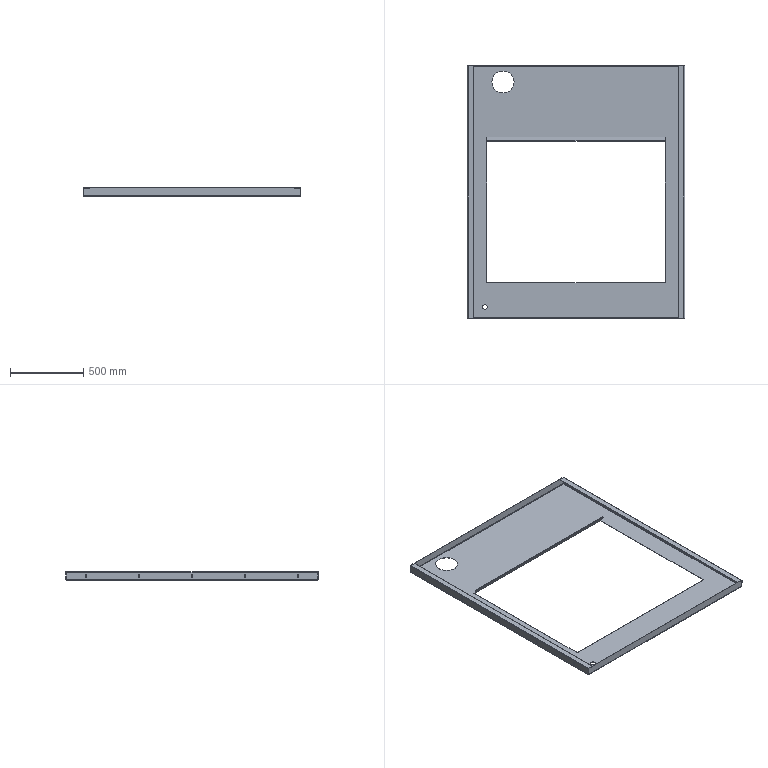Part | STEP file | SYL_0392D6J1SYL0380DJ10-1713006 | 1 solid | 150 faces | box 1478 x 1718 x 55 mm | volume 3668328 mm3 | plane 84 | cylinder 58 | spline 8 | commonest cylinder face diameters 10 x40 4 x7 8 x7 32 x2 150 x2